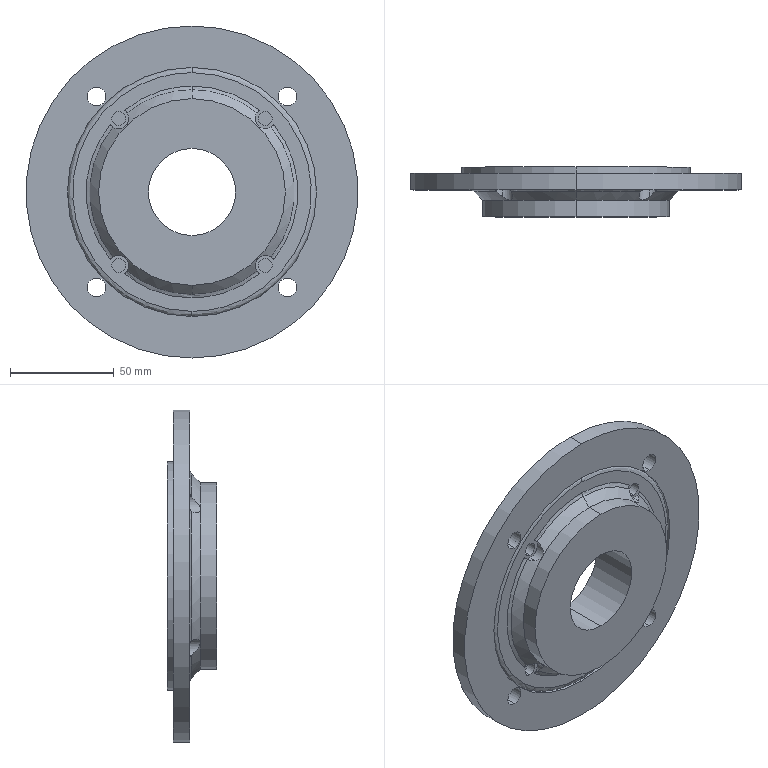Part | STEP file | PRODUCT_NAME_35_default | 1 solid | 50 faces | box 160 x 24 x 160 mm | volume 238568 mm3 | cylinder 32 | plane 9 | spline 7 | cone 2 | commonest cylinder face diameters 6.6 x8 9 x8 9.9 x6 42 x2 90 x2 110 x2